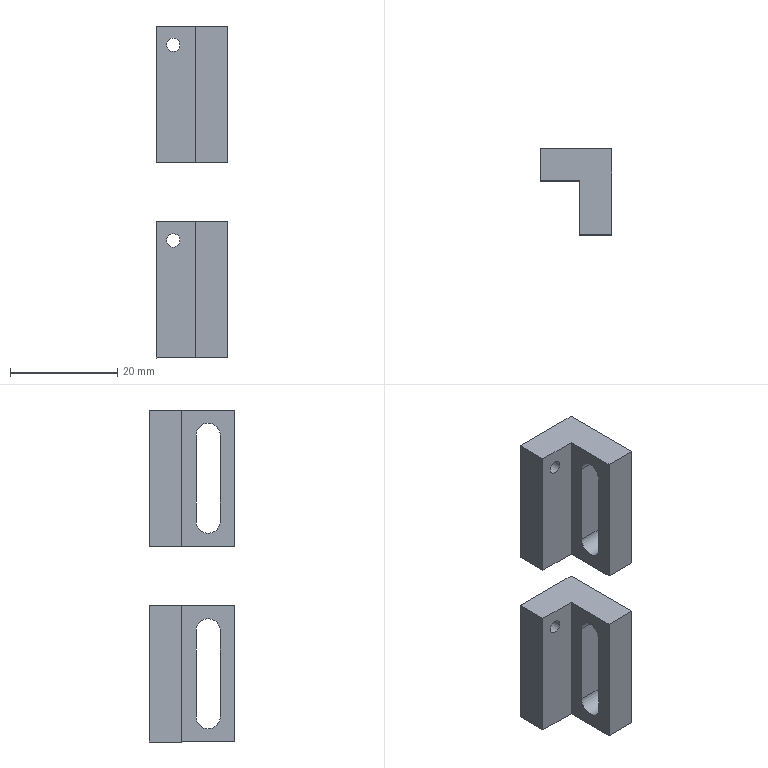Part | NX | 2 solids | 30 faces | box 13.4 x 16 x 61.8 mm | volume 5960 mm3 | plane 22 | cylinder 8 | commonest cylinder face diameters 2.5 x4 4.5 x4
STEP:
#1=CARTESIAN_POINT('',(208.55,31.5,174.1));
#2=VERTEX_POINT('',#1);
#3=CARTESIAN_POINT('',(207.3,31.5,174.1));
#4=DIRECTION('',(0.,-1.,0.));
#5=DIRECTION('',(1.,0.,0.));
#6=AXIS2_PLACEMENT_3D('',#3,#4,#5);
#7=CIRCLE('',#6,1.25);
#8=EDGE_CURVE('',#2,#2,#7,.T.);
#9=ORIENTED_EDGE('',*,*,#8,.F.);
#10=EDGE_LOOP('',(#9));
#11=FACE_BOUND('',#10,.T.);
#12=CARTESIAN_POINT('',(197.3,31.5,164.9));
#13=DIRECTION('',(0.,-1.,0.));
#14=DIRECTION('',(0.,0.,-1.));
#15=AXIS2_PLACEMENT_3D('',#12,#13,#14);
#16=PLANE('',#15);
#17=ADVANCED_FACE('',(#11),#16,.F.);
#18=CARTESIAN_POINT('',(208.55,37.5,174.1));
#19=VERTEX_POINT('',#18);
#20=CARTESIAN_POINT('',(207.3,37.5,174.1));
#21=DIRECTION('',(0.,-1.,0.));
#22=DIRECTION('',(1.,0.,0.));
#23=AXIS2_PLACEMENT_3D('',#20,#21,#22);
#24=CIRCLE('',#23,1.25);
#25=EDGE_CURVE('',#19,#19,#24,.T.);
#26=ORIENTED_EDGE('',*,*,#25,.T.);
#27=EDGE_LOOP('',(#26));
#28=FACE_BOUND('',#27,.T.);
#29=CARTESIAN_POINT('',(201.55,37.5,174.1));
#30=VERTEX_POINT('',#29);
#31=CARTESIAN_POINT('',(200.3,37.5,174.1));
#32=DIRECTION('',(0.,-1.,0.));
#33=DIRECTION('',(1.,0.,0.));
#34=AXIS2_PLACEMENT_3D('',#31,#32,#33);
#35=CIRCLE('',#34,1.25);
#36=EDGE_CURVE('',#30,#30,#35,.T.);
#37=ORIENTED_EDGE('',*,*,#36,.T.);
#38=EDGE_LOOP('',(#37));
#39=FACE_BOUND('',#38,.T.);
#40=CARTESIAN_POINT('',(197.1,37.5,177.6));
#41=VERTEX_POINT('',#40);
#42=CARTESIAN_POINT('',(197.1,37.5,152.2));
#43=VERTEX_POINT('',#42);
#44=CARTESIAN_POINT('',(197.1,37.5,177.6));
#45=DIRECTION('',(0.,0.,-1.));
#46=VECTOR('',#45,1000.);
#47=LINE('',#44,#46);
#48=EDGE_CURVE('',#41,#43,#47,.T.);
#49=ORIENTED_EDGE('',*,*,#48,.F.);
#50=CARTESIAN_POINT('',(210.5,37.5,177.6));
#51=VERTEX_POINT('',#50);
#52=CARTESIAN_POINT('',(203.5,37.5,177.6));
#53=DIRECTION('',(-1.,0.,0.));
#54=VECTOR('',#53,1000.);
#55=LINE('',#52,#54);
#56=EDGE_CURVE('',#51,#41,#55,.T.);
#57=ORIENTED_EDGE('',*,*,#56,.F.);
#58=CARTESIAN_POINT('',(210.5,37.5,152.2));
#59=VERTEX_POINT('',#58);
#60=CARTESIAN_POINT('',(210.5,37.5,164.9));
#61=DIRECTION('',(0.,0.,-1.));
#62=VECTOR('',#61,1000.);
#63=LINE('',#60,#62);
#64=EDGE_CURVE('',#51,#59,#63,.T.);
#65=ORIENTED_EDGE('',*,*,#64,.T.);
#66=CARTESIAN_POINT('',(203.5,37.5,152.2));
#67=DIRECTION('',(1.,0.,0.));
#68=VECTOR('',#67,1000.);
#69=LINE('',#66,#68);
#70=EDGE_CURVE('',#43,#59,#69,.T.);
#71=ORIENTED_EDGE('',*,*,#70,.F.);
#72=EDGE_LOOP('',(#49,#57,#65,#71));
#73=FACE_BOUND('',#72,.T.);
#74=CARTESIAN_POINT('',(196.8,37.5,164.9));
#75=DIRECTION('',(0.,1.,0.));
#76=DIRECTION('',(0.,0.,1.));
#77=AXIS2_PLACEMENT_3D('',#74,#75,#76);
#78=PLANE('',#77);
#79=ADVANCED_FACE('',(#28,#39,#73),#78,.T.);
#80=ORIENTED_EDGE('',*,*,#36,.F.);
#81=EDGE_LOOP('',(#80));
#82=FACE_BOUND('',#81,.T.);
#83=CARTESIAN_POINT('',(201.55,31.5,174.1));
#84=VERTEX_POINT('',#83);
#85=CARTESIAN_POINT('',(200.3,31.5,174.1));
#86=DIRECTION('',(0.,-1.,0.));
#87=DIRECTION('',(1.,0.,0.));
#88=AXIS2_PLACEMENT_3D('',#85,#86,#87);
#89=CIRCLE('',#88,1.25);
#90=EDGE_CURVE('',#84,#84,#89,.T.);
#91=ORIENTED_EDGE('',*,*,#90,.T.);
#92=EDGE_LOOP('',(#91));
#93=FACE_BOUND('',#92,.T.);
#94=CARTESIAN_POINT('',(200.3,31.5,174.1));
#95=DIRECTION('',(0.,1.,0.));
#96=DIRECTION('',(0.,0.,1.));
#97=AXIS2_PLACEMENT_3D('',#94,#95,#96);
#98=CYLINDRICAL_SURFACE('',#97,1.25);
#99=ADVANCED_FACE('',(#82,#93),#98,.F.);
#100=ORIENTED_EDGE('',*,*,#25,.F.);
#101=EDGE_LOOP('',(#100));
#102=FACE_BOUND('',#101,.T.);
#103=ORIENTED_EDGE('',*,*,#8,.T.);
#104=EDGE_LOOP('',(#103));
#105=FACE_BOUND('',#104,.T.);
#106=CARTESIAN_POINT('',(207.3,31.5,174.1));
#107=DIRECTION('',(0.,1.,0.));
#108=DIRECTION('',(0.,0.,1.));
#109=AXIS2_PLACEMENT_3D('',#106,#107,#108);
#110=CYLINDRICAL_SURFACE('',#109,1.25);
#111=ADVANCED_FACE('',(#102,#105),#110,.F.);
#112=CARTESIAN_POINT('',(197.1,31.5,177.6));
#113=VERTEX_POINT('',#112);
#114=CARTESIAN_POINT('',(197.1,31.5,152.2));
#115=VERTEX_POINT('',#114);
#116=CARTESIAN_POINT('',(197.1,31.5,164.9));
#117=DIRECTION('',(0.,0.,-1.));
#118=VECTOR('',#117,1000.);
#119=LINE('',#116,#118);
#120=EDGE_CURVE('',#113,#115,#119,.T.);
#121=ORIENTED_EDGE('',*,*,#120,.F.);
#122=CARTESIAN_POINT('',(197.1,31.5,177.6));
#123=DIRECTION('',(0.,1.,0.));
#124=VECTOR('',#123,1000.);
#125=LINE('',#122,#124);
#126=EDGE_CURVE('',#113,#41,#125,.T.);
#127=ORIENTED_EDGE('',*,*,#126,.T.);
#128=ORIENTED_EDGE('',*,*,#48,.T.);
#129=CARTESIAN_POINT('',(197.1,31.5,152.2));
#130=DIRECTION('',(0.,1.,0.));
#131=VECTOR('',#130,1000.);
#132=LINE('',#129,#131);
#133=EDGE_CURVE('',#115,#43,#132,.T.);
#134=ORIENTED_EDGE('',*,*,#133,.F.);
#135=EDGE_LOOP('',(#121,#127,#128,#134));
#136=FACE_BOUND('',#135,.T.);
#137=CARTESIAN_POINT('',(197.1,31.5,177.6));
#138=DIRECTION('',(-1.,0.,0.));
#139=DIRECTION('',(0.,0.,-1.));
#140=AXIS2_PLACEMENT_3D('',#137,#138,#139);
#141=PLANE('',#140);
#142=ADVANCED_FACE('',(#136),#141,.T.);
#143=CARTESIAN_POINT('',(204.5,31.5,152.2));
#144=VERTEX_POINT('',#143);
#145=CARTESIAN_POINT('',(197.3,31.5,152.2));
#146=DIRECTION('',(1.,0.,0.));
#147=VECTOR('',#146,1000.);
#148=LINE('',#145,#147);
#149=EDGE_CURVE('',#115,#144,#148,.T.);
#150=ORIENTED_EDGE('',*,*,#149,.T.);
#151=CARTESIAN_POINT('',(204.5,31.5,177.6));
#152=VERTEX_POINT('',#151);
#153=CARTESIAN_POINT('',(204.5,31.5,164.9));
#154=DIRECTION('',(0.,0.,1.));
#155=VECTOR('',#154,1000.);
#156=LINE('',#153,#155);
#157=EDGE_CURVE('',#144,#152,#156,.T.);
#158=ORIENTED_EDGE('',*,*,#157,.T.);
#159=CARTESIAN_POINT('',(197.3,31.5,177.6));
#160=DIRECTION('',(-1.,0.,0.));
#161=VECTOR('',#160,1000.);
#162=LINE('',#159,#161);
#163=EDGE_CURVE('',#152,#113,#162,.T.);
#164=ORIENTED_EDGE('',*,*,#163,.T.);
#165=ORIENTED_EDGE('',*,*,#120,.T.);
#166=EDGE_LOOP('',(#150,#158,#164,#165));
#167=FACE_BOUND('',#166,.T.);
#168=ORIENTED_EDGE('',*,*,#90,.F.);
#169=EDGE_LOOP('',(#168));
#170=FACE_BOUND('',#169,.T.);
#171=CARTESIAN_POINT('',(197.3,31.5,164.9));
#172=DIRECTION('',(0.,-1.,0.));
#173=DIRECTION('',(0.,0.,-1.));
#174=AXIS2_PLACEMENT_3D('',#171,#172,#173);
#175=PLANE('',#174);
#176=ADVANCED_FACE('',(#167,#170),#175,.T.);
#177=CARTESIAN_POINT('',(210.5,24.25,156.9));
#178=VERTEX_POINT('',#177);
#179=CARTESIAN_POINT('',(210.5,28.75,156.9));
#180=VERTEX_POINT('',#179);
#181=CARTESIAN_POINT('',(210.5,26.5,156.9));
#182=DIRECTION('',(1.,0.,0.));
#183=DIRECTION('',(0.,1.,0.));
#184=AXIS2_PLACEMENT_3D('',#181,#182,#183);
#185=CIRCLE('',#184,2.25);
#186=EDGE_CURVE('',#178,#180,#185,.T.);
#187=ORIENTED_EDGE('',*,*,#186,.F.);
#188=CARTESIAN_POINT('',(210.5,24.25,172.9));
#189=VERTEX_POINT('',#188);
#190=CARTESIAN_POINT('',(210.5,24.25,164.9));
#191=DIRECTION('',(0.,0.,1.));
#192=VECTOR('',#191,1000.);
#193=LINE('',#190,#192);
#194=EDGE_CURVE('',#178,#189,#193,.T.);
#195=ORIENTED_EDGE('',*,*,#194,.T.);
#196=CARTESIAN_POINT('',(210.5,28.75,172.9));
#197=VERTEX_POINT('',#196);
#198=CARTESIAN_POINT('',(210.5,26.5,172.9));
#199=DIRECTION('',(1.,0.,0.));
#200=DIRECTION('',(0.,1.,0.));
#201=AXIS2_PLACEMENT_3D('',#198,#199,#200);
#202=CIRCLE('',#201,2.25);
#203=EDGE_CURVE('',#197,#189,#202,.T.);
#204=ORIENTED_EDGE('',*,*,#203,.F.);
#205=CARTESIAN_POINT('',(210.5,28.75,164.9));
#206=DIRECTION('',(0.,0.,-1.));
#207=VECTOR('',#206,1000.);
#208=LINE('',#205,#207);
#209=EDGE_CURVE('',#197,#180,#208,.T.);
#210=ORIENTED_EDGE('',*,*,#209,.T.);
#211=EDGE_LOOP('',(#187,#195,#204,#210));
#212=FACE_BOUND('',#211,.T.);
#213=CARTESIAN_POINT('',(210.5,21.5,152.2));
#214=VERTEX_POINT('',#213);
#215=CARTESIAN_POINT('',(210.5,31.5,152.2));
#216=DIRECTION('',(0.,-1.,0.));
#217=VECTOR('',#216,1000.);
#218=LINE('',#215,#217);
#219=EDGE_CURVE('',#59,#214,#218,.T.);
#220=ORIENTED_EDGE('',*,*,#219,.F.);
#221=ORIENTED_EDGE('',*,*,#64,.F.);
#222=CARTESIAN_POINT('',(210.5,21.5,177.6));
#223=VERTEX_POINT('',#222);
#224=CARTESIAN_POINT('',(210.5,75.772,177.6));
#225=DIRECTION('',(0.,-1.,0.));
#226=VECTOR('',#225,1000.);
#227=LINE('',#224,#226);
#228=EDGE_CURVE('',#51,#223,#227,.T.);
#229=ORIENTED_EDGE('',*,*,#228,.T.);
#230=CARTESIAN_POINT('',(210.5,21.5,164.9));
#231=DIRECTION('',(0.,0.,-1.));
#232=VECTOR('',#231,1000.);
#233=LINE('',#230,#232);
#234=EDGE_CURVE('',#223,#214,#233,.T.);
#235=ORIENTED_EDGE('',*,*,#234,.T.);
#236=EDGE_LOOP('',(#220,#221,#229,#235));
#237=FACE_BOUND('',#236,.T.);
#238=CARTESIAN_POINT('',(210.5,75.772,167.4));
#239=DIRECTION('',(-1.,0.,0.));
#240=DIRECTION('',(0.,0.,-1.));
#241=AXIS2_PLACEMENT_3D('',#238,#239,#240);
#242=PLANE('',#241);
#243=ADVANCED_FACE('',(#212,#237),#242,.F.);
#244=ORIENTED_EDGE('',*,*,#228,.F.);
#245=ORIENTED_EDGE('',*,*,#56,.T.);
#246=ORIENTED_EDGE('',*,*,#126,.F.);
#247=ORIENTED_EDGE('',*,*,#163,.F.);
#248=CARTESIAN_POINT('',(204.5,21.5,177.6));
#249=VERTEX_POINT('',#248);
#250=CARTESIAN_POINT('',(204.5,31.5,177.6));
#251=DIRECTION('',(0.,1.,0.));
#252=VECTOR('',#251,1000.);
#253=LINE('',#250,#252);
#254=EDGE_CURVE('',#249,#152,#253,.T.);
#255=ORIENTED_EDGE('',*,*,#254,.F.);
#256=CARTESIAN_POINT('',(196.8,21.5,177.6));
#257=DIRECTION('',(-1.,0.,0.));
#258=VECTOR('',#257,1000.);
#259=LINE('',#256,#258);
#260=EDGE_CURVE('',#223,#249,#259,.T.);
#261=ORIENTED_EDGE('',*,*,#260,.F.);
#262=EDGE_LOOP('',(#244,#245,#246,#247,#255,#261));
#263=FACE_BOUND('',#262,.T.);
#264=CARTESIAN_POINT('',(203.5,31.5,177.6));
#265=DIRECTION('',(0.,0.,1.));
#266=DIRECTION('',(-1.,0.,0.));
#267=AXIS2_PLACEMENT_3D('',#264,#265,#266);
#268=PLANE('',#267);
#269=ADVANCED_FACE('',(#263),#268,.T.);
#270=CARTESIAN_POINT('',(204.5,21.5,152.2));
#271=VERTEX_POINT('',#270);
#272=CARTESIAN_POINT('',(204.5,31.5,152.2));
#273=DIRECTION('',(0.,-1.,0.));
#274=VECTOR('',#273,1000.);
#275=LINE('',#272,#274);
#276=EDGE_CURVE('',#144,#271,#275,.T.);
#277=ORIENTED_EDGE('',*,*,#276,.F.);
#278=ORIENTED_EDGE('',*,*,#149,.F.);
#279=ORIENTED_EDGE('',*,*,#133,.T.);
#280=ORIENTED_EDGE('',*,*,#70,.T.);
#281=ORIENTED_EDGE('',*,*,#219,.T.);
#282=CARTESIAN_POINT('',(196.8,21.5,152.2));
#283=DIRECTION('',(1.,0.,0.));
#284=VECTOR('',#283,1000.);
#285=LINE('',#282,#284);
#286=EDGE_CURVE('',#271,#214,#285,.T.);
#287=ORIENTED_EDGE('',*,*,#286,.F.);
#288=EDGE_LOOP('',(#277,#278,#279,#280,#281,#287));
#289=FACE_BOUND('',#288,.T.);
#290=CARTESIAN_POINT('',(203.5,31.5,152.2));
#291=DIRECTION('',(0.,0.,-1.));
#292=DIRECTION('',(1.,0.,0.));
#293=AXIS2_PLACEMENT_3D('',#290,#291,#292);
#294=PLANE('',#293);
#295=ADVANCED_FACE('',(#289),#294,.T.);
#296=ORIENTED_EDGE('',*,*,#276,.T.);
#297=CARTESIAN_POINT('',(204.5,21.5,164.9));
#298=DIRECTION('',(0.,0.,-1.));
#299=VECTOR('',#298,1000.);
#300=LINE('',#297,#299);
#301=EDGE_CURVE('',#249,#271,#300,.T.);
#302=ORIENTED_EDGE('',*,*,#301,.F.);
#303=ORIENTED_EDGE('',*,*,#254,.T.);
#304=ORIENTED_EDGE('',*,*,#157,.F.);
#305=EDGE_LOOP('',(#296,#302,#303,#304));
#306=FACE_BOUND('',#305,.T.);
#307=CARTESIAN_POINT('',(204.5,24.25,156.9));
#308=VERTEX_POINT('',#307);
#309=CARTESIAN_POINT('',(204.5,28.75,156.9));
#310=VERTEX_POINT('',#309);
#311=CARTESIAN_POINT('',(204.5,26.5,156.9));
#312=DIRECTION('',(1.,0.,0.));
#313=DIRECTION('',(0.,1.,0.));
#314=AXIS2_PLACEMENT_3D('',#311,#312,#313);
#315=CIRCLE('',#314,2.25);
#316=EDGE_CURVE('',#308,#310,#315,.T.);
#317=ORIENTED_EDGE('',*,*,#316,.T.);
#318=CARTESIAN_POINT('',(204.5,28.75,172.9));
#319=VERTEX_POINT('',#318);
#320=CARTESIAN_POINT('',(204.5,28.75,164.9));
#321=DIRECTION('',(0.,0.,-1.));
#322=VECTOR('',#321,1000.);
#323=LINE('',#320,#322);
#324=EDGE_CURVE('',#319,#310,#323,.T.);
#325=ORIENTED_EDGE('',*,*,#324,.F.);
#326=CARTESIAN_POINT('',(204.5,24.25,172.9));
#327=VERTEX_POINT('',#326);
#328=CARTESIAN_POINT('',(204.5,26.5,172.9));
#329=DIRECTION('',(1.,0.,0.));
#330=DIRECTION('',(0.,1.,0.));
#331=AXIS2_PLACEMENT_3D('',#328,#329,#330);
#332=CIRCLE('',#331,2.25);
#333=EDGE_CURVE('',#319,#327,#332,.T.);
#334=ORIENTED_EDGE('',*,*,#333,.T.);
#335=CARTESIAN_POINT('',(204.5,24.25,164.9));
#336=DIRECTION('',(0.,0.,1.));
#337=VECTOR('',#336,1000.);
#338=LINE('',#335,#337);
#339=EDGE_CURVE('',#308,#327,#338,.T.);
#340=ORIENTED_EDGE('',*,*,#339,.F.);
#341=EDGE_LOOP('',(#317,#325,#334,#340));
#342=FACE_BOUND('',#341,.T.);
#343=CARTESIAN_POINT('',(204.5,-81.728,177.4));
#344=DIRECTION('',(-1.,0.,0.));
#345=DIRECTION('',(0.,0.,-1.));
#346=AXIS2_PLACEMENT_3D('',#343,#344,#345);
#347=PLANE('',#346);
#348=ADVANCED_FACE('',(#306,#342),#347,.T.);
#349=CARTESIAN_POINT('',(210.5,24.25,156.9));
#350=DIRECTION('',(1.,0.,0.));
#351=VECTOR('',#350,1000.);
#352=LINE('',#349,#351);
#353=EDGE_CURVE('',#308,#178,#352,.T.);
#354=ORIENTED_EDGE('',*,*,#353,.T.);
#355=ORIENTED_EDGE('',*,*,#186,.T.);
#356=CARTESIAN_POINT('',(210.5,28.75,156.9));
#357=DIRECTION('',(-1.,0.,0.));
#358=VECTOR('',#357,1000.);
#359=LINE('',#356,#358);
#360=EDGE_CURVE('',#180,#310,#359,.T.);
#361=ORIENTED_EDGE('',*,*,#360,.T.);
#362=ORIENTED_EDGE('',*,*,#316,.F.);
#363=EDGE_LOOP('',(#354,#355,#361,#362));
#364=FACE_BOUND('',#363,.T.);
#365=CARTESIAN_POINT('',(210.5,26.5,156.9));
#366=DIRECTION('',(-1.,0.,0.));
#367=DIRECTION('',(0.,0.,-1.));
#368=AXIS2_PLACEMENT_3D('',#365,#366,#367);
#369=CYLINDRICAL_SURFACE('',#368,2.25);
#370=ADVANCED_FACE('',(#364),#369,.F.);
#371=ORIENTED_EDGE('',*,*,#324,.T.);
#372=ORIENTED_EDGE('',*,*,#360,.F.);
#373=ORIENTED_EDGE('',*,*,#209,.F.);
#374=CARTESIAN_POINT('',(210.5,28.75,172.9));
#375=DIRECTION('',(1.,0.,0.));
#376=VECTOR('',#375,1000.);
#377=LINE('',#374,#376);
#378=EDGE_CURVE('',#319,#197,#377,.T.);
#379=ORIENTED_EDGE('',*,*,#378,.F.);
#380=EDGE_LOOP('',(#371,#372,#373,#379));
#381=FACE_BOUND('',#380,.T.);
#382=CARTESIAN_POINT('',(210.5,28.75,164.9));
#383=DIRECTION('',(0.,1.,0.));
#384=DIRECTION('',(0.,0.,1.));
#385=AXIS2_PLACEMENT_3D('',#382,#383,#384);
#386=PLANE('',#385);
#387=ADVANCED_FACE('',(#381),#386,.F.);
#388=ORIENTED_EDGE('',*,*,#378,.T.);
#389=ORIENTED_EDGE('',*,*,#203,.T.);
#390=CARTESIAN_POINT('',(210.5,24.25,172.9));
#391=DIRECTION('',(-1.,0.,0.));
#392=VECTOR('',#391,1000.);
#393=LINE('',#390,#392);
#394=EDGE_CURVE('',#189,#327,#393,.T.);
#395=ORIENTED_EDGE('',*,*,#394,.T.);
#396=ORIENTED_EDGE('',*,*,#333,.F.);
#397=EDGE_LOOP('',(#388,#389,#395,#396));
#398=FACE_BOUND('',#397,.T.);
#399=CARTESIAN_POINT('',(210.5,26.5,172.9));
#400=DIRECTION('',(-1.,0.,0.));
#401=DIRECTION('',(0.,0.,-1.));
#402=AXIS2_PLACEMENT_3D('',#399,#400,#401);
#403=CYLINDRICAL_SURFACE('',#402,2.25);
#404=ADVANCED_FACE('',(#398),#403,.F.);
#405=ORIENTED_EDGE('',*,*,#194,.F.);
#406=ORIENTED_EDGE('',*,*,#353,.F.);
#407=ORIENTED_EDGE('',*,*,#339,.T.);
#408=ORIENTED_EDGE('',*,*,#394,.F.);
#409=EDGE_LOOP('',(#405,#406,#407,#408));
#410=FACE_BOUND('',#409,.T.);
#411=CARTESIAN_POINT('',(210.5,24.25,164.9));
#412=DIRECTION('',(0.,-1.,0.));
#413=DIRECTION('',(0.,0.,-1.));
#414=AXIS2_PLACEMENT_3D('',#411,#412,#413);
#415=PLANE('',#414);
#416=ADVANCED_FACE('',(#410),#415,.F.);
#417=ORIENTED_EDGE('',*,*,#301,.T.);
#418=ORIENTED_EDGE('',*,*,#286,.T.);
#419=ORIENTED_EDGE('',*,*,#234,.F.);
#420=ORIENTED_EDGE('',*,*,#260,.T.);
#421=EDGE_LOOP('',(#417,#418,#419,#420));
#422=FACE_BOUND('',#421,.T.);
#423=CARTESIAN_POINT('',(196.8,21.5,164.9));
#424=DIRECTION('',(0.,1.,0.));
#425=DIRECTION('',(0.,0.,1.));
#426=AXIS2_PLACEMENT_3D('',#423,#424,#425);
#427=PLANE('',#426);
#428=ADVANCED_FACE('',(#422),#427,.F.);
#429=CLOSED_SHELL('',(#17,#79,#99,#111,#142,#176,#243,#269,#295,#348,#370,#387,#404,#416,#428));
#430=MANIFOLD_SOLID_BREP('',#429);
#431=CARTESIAN_POINT('',(208.55,31.5,137.7));
#432=VERTEX_POINT('',#431);
#433=CARTESIAN_POINT('',(207.3,31.5,137.7));
#434=DIRECTION('',(0.,-1.,0.));
#435=DIRECTION('',(1.,0.,0.));
#436=AXIS2_PLACEMENT_3D('',#433,#434,#435);
#437=CIRCLE('',#436,1.25);
#438=EDGE_CURVE('',#432,#432,#437,.T.);
#439=ORIENTED_EDGE('',*,*,#438,.F.);
#440=EDGE_LOOP('',(#439));
#441=FACE_BOUND('',#440,.T.);
#442=CARTESIAN_POINT('',(197.3,31.5,128.5));
#443=DIRECTION('',(0.,-1.,0.));
#444=DIRECTION('',(0.,0.,-1.));
#445=AXIS2_PLACEMENT_3D('',#442,#443,#444);
#446=PLANE('',#445);
#447=ADVANCED_FACE('',(#441),#446,.F.);
#448=CARTESIAN_POINT('',(208.55,37.5,137.7));
#449=VERTEX_POINT('',#448);
#450=CARTESIAN_POINT('',(207.3,37.5,137.7));
#451=DIRECTION('',(0.,-1.,0.));
#452=DIRECTION('',(1.,0.,0.));
#453=AXIS2_PLACEMENT_3D('',#450,#451,#452);
#454=CIRCLE('',#453,1.25);
#455=EDGE_CURVE('',#449,#449,#454,.T.);
#456=ORIENTED_EDGE('',*,*,#455,.T.);
#457=EDGE_LOOP('',(#456));
#458=FACE_BOUND('',#457,.T.);
#459=CARTESIAN_POINT('',(201.55,37.5,137.7));
#460=VERTEX_POINT('',#459);
#461=CARTESIAN_POINT('',(200.3,37.5,137.7));
#462=DIRECTION('',(0.,-1.,0.));
#463=DIRECTION('',(1.,0.,0.));
#464=AXIS2_PLACEMENT_3D('',#461,#462,#463);
#465=CIRCLE('',#464,1.25);
#466=EDGE_CURVE('',#460,#460,#465,.T.);
#467=ORIENTED_EDGE('',*,*,#466,.T.);
#468=EDGE_LOOP('',(#467));
#469=FACE_BOUND('',#468,.T.);
#470=CARTESIAN_POINT('',(197.1,37.5,141.2));
#471=VERTEX_POINT('',#470);
#472=CARTESIAN_POINT('',(197.1,37.5,115.8));
#473=VERTEX_POINT('',#472);
#474=CARTESIAN_POINT('',(197.1,37.5,141.2));
#475=DIRECTION('',(0.,0.,-1.));
#476=VECTOR('',#475,1000.);
#477=LINE('',#474,#476);
#478=EDGE_CURVE('',#471,#473,#477,.T.);
#479=ORIENTED_EDGE('',*,*,#478,.F.);
#480=CARTESIAN_POINT('',(210.5,37.5,141.2));
#481=VERTEX_POINT('',#480);
#482=CARTESIAN_POINT('',(203.5,37.5,141.2));
#483=DIRECTION('',(-1.,0.,0.));
#484=VECTOR('',#483,1000.);
#485=LINE('',#482,#484);
#486=EDGE_CURVE('',#481,#471,#485,.T.);
#487=ORIENTED_EDGE('',*,*,#486,.F.);
#488=CARTESIAN_POINT('',(210.5,37.5,115.8));
#489=VERTEX_POINT('',#488);
#490=CARTESIAN_POINT('',(210.5,37.5,128.5));
#491=DIRECTION('',(0.,0.,-1.));
#492=VECTOR('',#491,1000.);
#493=LINE('',#490,#492);
#494=EDGE_CURVE('',#481,#489,#493,.T.);
#495=ORIENTED_EDGE('',*,*,#494,.T.);
#496=CARTESIAN_POINT('',(203.5,37.5,115.8));
#497=DIRECTION('',(1.,0.,0.));
#498=VECTOR('',#497,1000.);
#499=LINE('',#496,#498);
#500=EDGE_CURVE('',#473,#489,#499,.T.);
#501=ORIENTED_EDGE('',*,*,#500,.F.);
#502=EDGE_LOOP('',(#479,#487,#495,#501));
#503=FACE_BOUND('',#502,.T.);
#504=CARTESIAN_POINT('',(196.8,37.5,128.5));
#505=DIRECTION('',(0.,1.,0.));
#506=DIRECTION('',(0.,0.,1.));
#507=AXIS2_PLACEMENT_3D('',#504,#505,#506);
#508=PLANE('',#507);
#509=ADVANCED_FACE('',(#458,#469,#503),#508,.T.);
#510=ORIENTED_EDGE('',*,*,#466,.F.);
#511=EDGE_LOOP('',(#510));
#512=FACE_BOUND('',#511,.T.);
#513=CARTESIAN_POINT('',(201.55,31.5,137.7));
#514=VERTEX_POINT('',#513);
#515=CARTESIAN_POINT('',(200.3,31.5,137.7));
#516=DIRECTION('',(0.,-1.,0.));
#517=DIRECTION('',(1.,0.,0.));
#518=AXIS2_PLACEMENT_3D('',#515,#516,#517);
#519=CIRCLE('',#518,1.25);
#520=EDGE_CURVE('',#514,#514,#519,.T.);
#521=ORIENTED_EDGE('',*,*,#520,.T.);
#522=EDGE_LOOP('',(#521));
#523=FACE_BOUND('',#522,.T.);
#524=CARTESIAN_POINT('',(200.3,31.5,137.7));
#525=DIRECTION('',(0.,1.,0.));
#526=DIRECTION('',(0.,0.,1.));
#527=AXIS2_PLACEMENT_3D('',#524,#525,#526);
#528=CYLINDRICAL_SURFACE('',#527,1.25);
#529=ADVANCED_FACE('',(#512,#523),#528,.F.);
#530=ORIENTED_EDGE('',*,*,#455,.F.);
#531=EDGE_LOOP('',(#530));
#532=FACE_BOUND('',#531,.T.);
#533=ORIENTED_EDGE('',*,*,#438,.T.);
#534=EDGE_LOOP('',(#533));
#535=FACE_BOUND('',#534,.T.);
#536=CARTESIAN_POINT('',(207.3,31.5,137.7));
#537=DIRECTION('',(0.,1.,0.));
#538=DIRECTION('',(0.,0.,1.));
#539=AXIS2_PLACEMENT_3D('',#536,#537,#538);
#540=CYLINDRICAL_SURFACE('',#539,1.25);
#541=ADVANCED_FACE('',(#532,#535),#540,.F.);
#542=CARTESIAN_POINT('',(197.1,31.5,141.2));
#543=VERTEX_POINT('',#542);
#544=CARTESIAN_POINT('',(197.1,31.5,115.8));
#545=VERTEX_POINT('',#544);
#546=CARTESIAN_POINT('',(197.1,31.5,128.5));
#547=DIRECTION('',(0.,0.,-1.));
#548=VECTOR('',#547,1000.);
#549=LINE('',#546,#548);
#550=EDGE_CURVE('',#543,#545,#549,.T.);
#551=ORIENTED_EDGE('',*,*,#550,.F.);
#552=CARTESIAN_POINT('',(197.1,31.5,141.2));
#553=DIRECTION('',(0.,1.,0.));
#554=VECTOR('',#553,1000.);
#555=LINE('',#552,#554);
#556=EDGE_CURVE('',#543,#471,#555,.T.);
#557=ORIENTED_EDGE('',*,*,#556,.T.);
#558=ORIENTED_EDGE('',*,*,#478,.T.);
#559=CARTESIAN_POINT('',(197.1,31.5,115.8));
#560=DIRECTION('',(0.,1.,0.));
#561=VECTOR('',#560,1000.);
#562=LINE('',#559,#561);
#563=EDGE_CURVE('',#545,#473,#562,.T.);
#564=ORIENTED_EDGE('',*,*,#563,.F.);
#565=EDGE_LOOP('',(#551,#557,#558,#564));
#566=FACE_BOUND('',#565,.T.);
#567=CARTESIAN_POINT('',(197.1,31.5,141.2));
#568=DIRECTION('',(-1.,0.,0.));
#569=DIRECTION('',(0.,0.,-1.));
#570=AXIS2_PLACEMENT_3D('',#567,#568,#569);
#571=PLANE('',#570);
#572=ADVANCED_FACE('',(#566),#571,.T.);
#573=CARTESIAN_POINT('',(204.5,31.5,115.8));
#574=VERTEX_POINT('',#573);
#575=CARTESIAN_POINT('',(197.3,31.5,115.8));
#576=DIRECTION('',(1.,0.,0.));
#577=VECTOR('',#576,1000.);
#578=LINE('',#575,#577);
#579=EDGE_CURVE('',#545,#574,#578,.T.);
#580=ORIENTED_EDGE('',*,*,#579,.T.);
#581=CARTESIAN_POINT('',(204.5,31.5,141.2));
#582=VERTEX_POINT('',#581);
#583=CARTESIAN_POINT('',(204.5,31.5,128.5));
#584=DIRECTION('',(0.,0.,1.));
#585=VECTOR('',#584,1000.);
#586=LINE('',#583,#585);
#587=EDGE_CURVE('',#574,#582,#586,.T.);
#588=ORIENTED_EDGE('',*,*,#587,.T.);
#589=CARTESIAN_POINT('',(197.3,31.5,141.2));
#590=DIRECTION('',(-1.,0.,0.));
#591=VECTOR('',#590,1000.);
#592=LINE('',#589,#591);
#593=EDGE_CURVE('',#582,#543,#592,.T.);
#594=ORIENTED_EDGE('',*,*,#593,.T.);
#595=ORIENTED_EDGE('',*,*,#550,.T.);
#596=EDGE_LOOP('',(#580,#588,#594,#595));
#597=FACE_BOUND('',#596,.T.);
#598=ORIENTED_EDGE('',*,*,#520,.F.);
#599=EDGE_LOOP('',(#598));
#600=FACE_BOUND('',#599,.T.);
#601=CARTESIAN_POINT('',(197.3,31.5,128.5));
#602=DIRECTION('',(0.,-1.,0.));
#603=DIRECTION('',(0.,0.,-1.));
#604=AXIS2_PLACEMENT_3D('',#601,#602,#603);
#605=PLANE('',#604);
#606=ADVANCED_FACE('',(#597,#600),#605,.T.);
#607=CARTESIAN_POINT('',(210.5,24.25,120.5));
#608=VERTEX_POINT('',#607);
#609=CARTESIAN_POINT('',(210.5,28.75,120.5));
#610=VERTEX_POINT('',#609);
#611=CARTESIAN_POINT('',(210.5,26.5,120.5));
#612=DIRECTION('',(1.,0.,0.));
#613=DIRECTION('',(0.,1.,0.));
#614=AXIS2_PLACEMENT_3D('',#611,#612,#613);
#615=CIRCLE('',#614,2.25);
#616=EDGE_CURVE('',#608,#610,#615,.T.);
#617=ORIENTED_EDGE('',*,*,#616,.F.);
#618=CARTESIAN_POINT('',(210.5,24.25,136.5));
#619=VERTEX_POINT('',#618);
#620=CARTESIAN_POINT('',(210.5,24.25,128.5));
#621=DIRECTION('',(0.,0.,1.));
#622=VECTOR('',#621,1000.);
#623=LINE('',#620,#622);
#624=EDGE_CURVE('',#608,#619,#623,.T.);
#625=ORIENTED_EDGE('',*,*,#624,.T.);
#626=CARTESIAN_POINT('',(210.5,28.75,136.5));
#627=VERTEX_POINT('',#626);
#628=CARTESIAN_POINT('',(210.5,26.5,136.5));
#629=DIRECTION('',(1.,0.,0.));
#630=DIRECTION('',(0.,1.,0.));
#631=AXIS2_PLACEMENT_3D('',#628,#629,#630);
#632=CIRCLE('',#631,2.25);
#633=EDGE_CURVE('',#627,#619,#632,.T.);
#634=ORIENTED_EDGE('',*,*,#633,.F.);
#635=CARTESIAN_POINT('',(210.5,28.75,128.5));
#636=DIRECTION('',(0.,0.,-1.));
#637=VECTOR('',#636,1000.);
#638=LINE('',#635,#637);
#639=EDGE_CURVE('',#627,#610,#638,.T.);
#640=ORIENTED_EDGE('',*,*,#639,.T.);
#641=EDGE_LOOP('',(#617,#625,#634,#640));
#642=FACE_BOUND('',#641,.T.);
#643=CARTESIAN_POINT('',(210.5,21.5,115.8));
#644=VERTEX_POINT('',#643);
#645=CARTESIAN_POINT('',(210.5,31.5,115.8));
#646=DIRECTION('',(0.,-1.,0.));
#647=VECTOR('',#646,1000.);
#648=LINE('',#645,#647);
#649=EDGE_CURVE('',#489,#644,#648,.T.);
#650=ORIENTED_EDGE('',*,*,#649,.F.);
#651=ORIENTED_EDGE('',*,*,#494,.F.);
#652=CARTESIAN_POINT('',(210.5,21.5,141.2));
#653=VERTEX_POINT('',#652);
#654=CARTESIAN_POINT('',(210.5,75.772,141.2));
#655=DIRECTION('',(0.,-1.,0.));
#656=VECTOR('',#655,1000.);
#657=LINE('',#654,#656);
#658=EDGE_CURVE('',#481,#653,#657,.T.);
#659=ORIENTED_EDGE('',*,*,#658,.T.);
#660=CARTESIAN_POINT('',(210.5,21.5,128.5));
#661=DIRECTION('',(0.,0.,-1.));
#662=VECTOR('',#661,1000.);
#663=LINE('',#660,#662);
#664=EDGE_CURVE('',#653,#644,#663,.T.);
#665=ORIENTED_EDGE('',*,*,#664,.T.);
#666=EDGE_LOOP('',(#650,#651,#659,#665));
#667=FACE_BOUND('',#666,.T.);
#668=CARTESIAN_POINT('',(210.5,75.772,131.));
#669=DIRECTION('',(-1.,0.,0.));
#670=DIRECTION('',(0.,0.,-1.));
#671=AXIS2_PLACEMENT_3D('',#668,#669,#670);
#672=PLANE('',#671);
#673=ADVANCED_FACE('',(#642,#667),#672,.F.);
#674=ORIENTED_EDGE('',*,*,#658,.F.);
#675=ORIENTED_EDGE('',*,*,#486,.T.);
#676=ORIENTED_EDGE('',*,*,#556,.F.);
#677=ORIENTED_EDGE('',*,*,#593,.F.);
#678=CARTESIAN_POINT('',(204.5,21.5,141.2));
#679=VERTEX_POINT('',#678);
#680=CARTESIAN_POINT('',(204.5,31.5,141.2));
#681=DIRECTION('',(0.,1.,0.));
#682=VECTOR('',#681,1000.);
#683=LINE('',#680,#682);
#684=EDGE_CURVE('',#679,#582,#683,.T.);
#685=ORIENTED_EDGE('',*,*,#684,.F.);
#686=CARTESIAN_POINT('',(196.8,21.5,141.2));
#687=DIRECTION('',(-1.,0.,0.));
#688=VECTOR('',#687,1000.);
#689=LINE('',#686,#688);
#690=EDGE_CURVE('',#653,#679,#689,.T.);
#691=ORIENTED_EDGE('',*,*,#690,.F.);
#692=EDGE_LOOP('',(#674,#675,#676,#677,#685,#691));
#693=FACE_BOUND('',#692,.T.);
#694=CARTESIAN_POINT('',(203.5,31.5,141.2));
#695=DIRECTION('',(0.,0.,1.));
#696=DIRECTION('',(-1.,0.,0.));
#697=AXIS2_PLACEMENT_3D('',#694,#695,#696);
#698=PLANE('',#697);
#699=ADVANCED_FACE('',(#693),#698,.T.);
#700=CARTESIAN_POINT('',(204.5,21.5,115.8));
#701=VERTEX_POINT('',#700);
#702=CARTESIAN_POINT('',(204.5,31.5,115.8));
#703=DIRECTION('',(0.,-1.,0.));
#704=VECTOR('',#703,1000.);
#705=LINE('',#702,#704);
#706=EDGE_CURVE('',#574,#701,#705,.T.);
#707=ORIENTED_EDGE('',*,*,#706,.F.);
#708=ORIENTED_EDGE('',*,*,#579,.F.);
#709=ORIENTED_EDGE('',*,*,#563,.T.);
#710=ORIENTED_EDGE('',*,*,#500,.T.);
#711=ORIENTED_EDGE('',*,*,#649,.T.);
#712=CARTESIAN_POINT('',(196.8,21.5,115.8));
#713=DIRECTION('',(1.,0.,0.));
#714=VECTOR('',#713,1000.);
#715=LINE('',#712,#714);
#716=EDGE_CURVE('',#701,#644,#715,.T.);
#717=ORIENTED_EDGE('',*,*,#716,.F.);
#718=EDGE_LOOP('',(#707,#708,#709,#710,#711,#717));
#719=FACE_BOUND('',#718,.T.);
#720=CARTESIAN_POINT('',(203.5,31.5,115.8));
#721=DIRECTION('',(0.,0.,-1.));
#722=DIRECTION('',(1.,0.,0.));
#723=AXIS2_PLACEMENT_3D('',#720,#721,#722);
#724=PLANE('',#723);
#725=ADVANCED_FACE('',(#719),#724,.T.);
#726=ORIENTED_EDGE('',*,*,#706,.T.);
#727=CARTESIAN_POINT('',(204.5,21.5,128.5));
#728=DIRECTION('',(0.,0.,-1.));
#729=VECTOR('',#728,1000.);
#730=LINE('',#727,#729);
#731=EDGE_CURVE('',#679,#701,#730,.T.);
#732=ORIENTED_EDGE('',*,*,#731,.F.);
#733=ORIENTED_EDGE('',*,*,#684,.T.);
#734=ORIENTED_EDGE('',*,*,#587,.F.);
#735=EDGE_LOOP('',(#726,#732,#733,#734));
#736=FACE_BOUND('',#735,.T.);
#737=CARTESIAN_POINT('',(204.5,24.25,120.5));
#738=VERTEX_POINT('',#737);
#739=CARTESIAN_POINT('',(204.5,28.75,120.5));
#740=VERTEX_POINT('',#739);
#741=CARTESIAN_POINT('',(204.5,26.5,120.5));
#742=DIRECTION('',(1.,0.,0.));
#743=DIRECTION('',(0.,1.,0.));
#744=AXIS2_PLACEMENT_3D('',#741,#742,#743);
#745=CIRCLE('',#744,2.25);
#746=EDGE_CURVE('',#738,#740,#745,.T.);
#747=ORIENTED_EDGE('',*,*,#746,.T.);
#748=CARTESIAN_POINT('',(204.5,28.75,136.5));
#749=VERTEX_POINT('',#748);
#750=CARTESIAN_POINT('',(204.5,28.75,128.5));
#751=DIRECTION('',(0.,0.,-1.));
#752=VECTOR('',#751,1000.);
#753=LINE('',#750,#752);
#754=EDGE_CURVE('',#749,#740,#753,.T.);
#755=ORIENTED_EDGE('',*,*,#754,.F.);
#756=CARTESIAN_POINT('',(204.5,24.25,136.5));
#757=VERTEX_POINT('',#756);
#758=CARTESIAN_POINT('',(204.5,26.5,136.5));
#759=DIRECTION('',(1.,0.,0.));
#760=DIRECTION('',(0.,1.,0.));
#761=AXIS2_PLACEMENT_3D('',#758,#759,#760);
#762=CIRCLE('',#761,2.25);
#763=EDGE_CURVE('',#749,#757,#762,.T.);
#764=ORIENTED_EDGE('',*,*,#763,.T.);
#765=CARTESIAN_POINT('',(204.5,24.25,128.5));
#766=DIRECTION('',(0.,0.,1.));
#767=VECTOR('',#766,1000.);
#768=LINE('',#765,#767);
#769=EDGE_CURVE('',#738,#757,#768,.T.);
#770=ORIENTED_EDGE('',*,*,#769,.F.);
#771=EDGE_LOOP('',(#747,#755,#764,#770));
#772=FACE_BOUND('',#771,.T.);
#773=CARTESIAN_POINT('',(204.5,-81.728,141.));
#774=DIRECTION('',(-1.,0.,0.));
#775=DIRECTION('',(0.,0.,-1.));
#776=AXIS2_PLACEMENT_3D('',#773,#774,#775);
#777=PLANE('',#776);
#778=ADVANCED_FACE('',(#736,#772),#777,.T.);
#779=CARTESIAN_POINT('',(210.5,24.25,120.5));
#780=DIRECTION('',(1.,0.,0.));
#781=VECTOR('',#780,1000.);
#782=LINE('',#779,#781);
#783=EDGE_CURVE('',#738,#608,#782,.T.);
#784=ORIENTED_EDGE('',*,*,#783,.T.);
#785=ORIENTED_EDGE('',*,*,#616,.T.);
#786=CARTESIAN_POINT('',(210.5,28.75,120.5));
#787=DIRECTION('',(-1.,0.,0.));
#788=VECTOR('',#787,1000.);
#789=LINE('',#786,#788);
#790=EDGE_CURVE('',#610,#740,#789,.T.);
#791=ORIENTED_EDGE('',*,*,#790,.T.);
#792=ORIENTED_EDGE('',*,*,#746,.F.);
#793=EDGE_LOOP('',(#784,#785,#791,#792));
#794=FACE_BOUND('',#793,.T.);
#795=CARTESIAN_POINT('',(210.5,26.5,120.5));
#796=DIRECTION('',(-1.,0.,0.));
#797=DIRECTION('',(0.,0.,-1.));
#798=AXIS2_PLACEMENT_3D('',#795,#796,#797);
#799=CYLINDRICAL_SURFACE('',#798,2.25);
#800=ADVANCED_FACE('',(#794),#799,.F.);
#801=ORIENTED_EDGE('',*,*,#754,.T.);
#802=ORIENTED_EDGE('',*,*,#790,.F.);
#803=ORIENTED_EDGE('',*,*,#639,.F.);
#804=CARTESIAN_POINT('',(210.5,28.75,136.5));
#805=DIRECTION('',(1.,0.,0.));
#806=VECTOR('',#805,1000.);
#807=LINE('',#804,#806);
#808=EDGE_CURVE('',#749,#627,#807,.T.);
#809=ORIENTED_EDGE('',*,*,#808,.F.);
#810=EDGE_LOOP('',(#801,#802,#803,#809));
#811=FACE_BOUND('',#810,.T.);
#812=CARTESIAN_POINT('',(210.5,28.75,128.5));
#813=DIRECTION('',(0.,1.,0.));
#814=DIRECTION('',(0.,0.,1.));
#815=AXIS2_PLACEMENT_3D('',#812,#813,#814);
#816=PLANE('',#815);
#817=ADVANCED_FACE('',(#811),#816,.F.);
#818=ORIENTED_EDGE('',*,*,#808,.T.);
#819=ORIENTED_EDGE('',*,*,#633,.T.);
#820=CARTESIAN_POINT('',(210.5,24.25,136.5));
#821=DIRECTION('',(-1.,0.,0.));
#822=VECTOR('',#821,1000.);
#823=LINE('',#820,#822);
#824=EDGE_CURVE('',#619,#757,#823,.T.);
#825=ORIENTED_EDGE('',*,*,#824,.T.);
#826=ORIENTED_EDGE('',*,*,#763,.F.);
#827=EDGE_LOOP('',(#818,#819,#825,#826));
#828=FACE_BOUND('',#827,.T.);
#829=CARTESIAN_POINT('',(210.5,26.5,136.5));
#830=DIRECTION('',(-1.,0.,0.));
#831=DIRECTION('',(0.,0.,-1.));
#832=AXIS2_PLACEMENT_3D('',#829,#830,#831);
#833=CYLINDRICAL_SURFACE('',#832,2.25);
#834=ADVANCED_FACE('',(#828),#833,.F.);
#835=ORIENTED_EDGE('',*,*,#624,.F.);
#836=ORIENTED_EDGE('',*,*,#783,.F.);
#837=ORIENTED_EDGE('',*,*,#769,.T.);
#838=ORIENTED_EDGE('',*,*,#824,.F.);
#839=EDGE_LOOP('',(#835,#836,#837,#838));
#840=FACE_BOUND('',#839,.T.);
#841=CARTESIAN_POINT('',(210.5,24.25,128.5));
#842=DIRECTION('',(0.,-1.,0.));
#843=DIRECTION('',(0.,0.,-1.));
#844=AXIS2_PLACEMENT_3D('',#841,#842,#843);
#845=PLANE('',#844);
#846=ADVANCED_FACE('',(#840),#845,.F.);
#847=ORIENTED_EDGE('',*,*,#731,.T.);
#848=ORIENTED_EDGE('',*,*,#716,.T.);
#849=ORIENTED_EDGE('',*,*,#664,.F.);
#850=ORIENTED_EDGE('',*,*,#690,.T.);
#851=EDGE_LOOP('',(#847,#848,#849,#850));
#852=FACE_BOUND('',#851,.T.);
#853=CARTESIAN_POINT('',(196.8,21.5,128.5));
#854=DIRECTION('',(0.,1.,0.));
#855=DIRECTION('',(0.,0.,1.));
#856=AXIS2_PLACEMENT_3D('',#853,#854,#855);
#857=PLANE('',#856);
#858=ADVANCED_FACE('',(#852),#857,.F.);
#859=CLOSED_SHELL('',(#447,#509,#529,#541,#572,#606,#673,#699,#725,#778,#800,#817,#834,#846,#858));
#860=MANIFOLD_SOLID_BREP('',#859);
#861=(LENGTH_UNIT()NAMED_UNIT(*)SI_UNIT(.MILLI.,.METRE.));
#862=UNCERTAINTY_MEASURE_WITH_UNIT(LENGTH_MEASURE(0.00001),#861,'','');
#863=(NAMED_UNIT(*)PLANE_ANGLE_UNIT()SI_UNIT($,.RADIAN.));
#864=(NAMED_UNIT(*)SI_UNIT($,.STERADIAN.)SOLID_ANGLE_UNIT());
#865=(GEOMETRIC_REPRESENTATION_CONTEXT(3)GLOBAL_UNCERTAINTY_ASSIGNED_CONTEXT((#862))GLOBAL_UNIT_ASSIGNED_CONTEXT((#861,#863,#864))REPRESENTATION_CONTEXT('',''));
#866=ADVANCED_BREP_SHAPE_REPRESENTATION('',(#430,#860),#865);